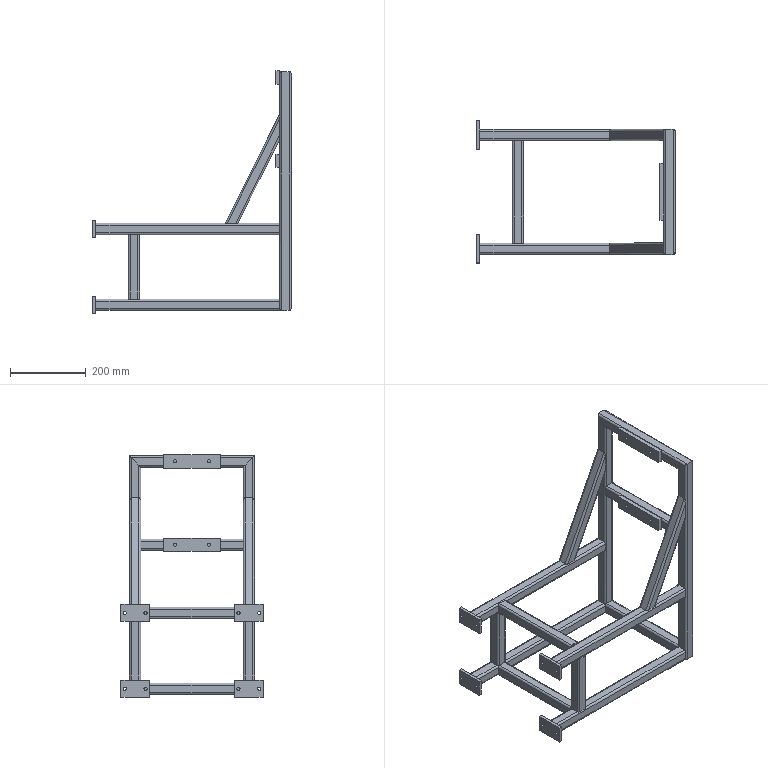Part | SolidWorks | features WeldCornerFeat 4, HoleWzd 2, ICE 2, 3DProfileFeature 1, WeldMemberFeat 1, WeldmentFeature 1 | 21 solids | 338 faces | box 523 x 375 x 640 mm | volume 1667392 mm3 | plane 186 | cylinder 152 | commonest cylinder face diameters 5.2 x60 10.4 x60 8.5 x32